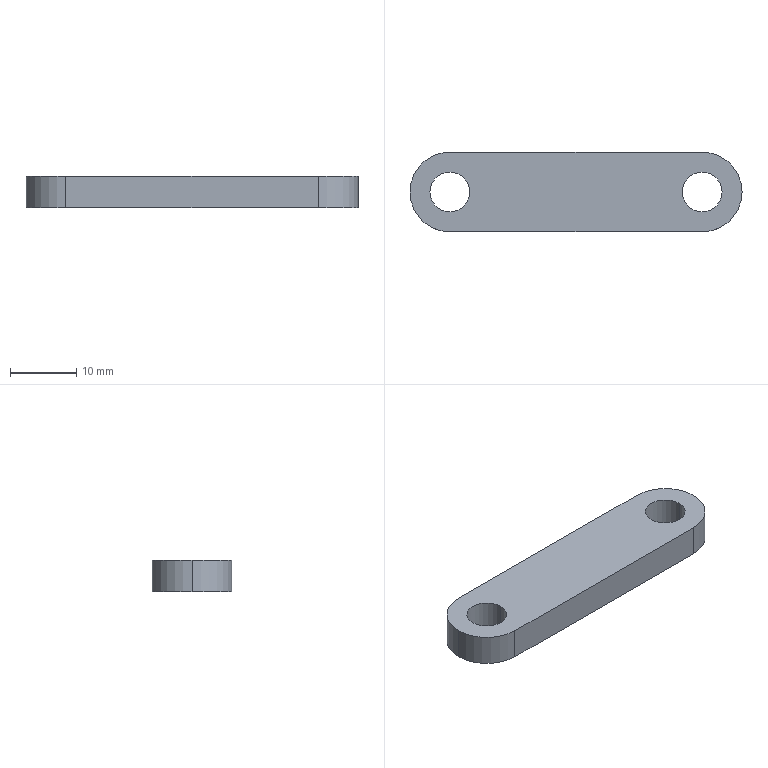Part | STEP file | Ngam kep 5 | 1 solid | 12 faces | box 50 x 12 x 4.8 mm | volume 2460 mm3 | cylinder 8 | plane 4 | commonest cylinder face diameters 6 x4 12 x4
STEP:
#1=CARTESIAN_POINT('',(0.,0.,0.));
#2=DIRECTION('',(0.,0.,1.));
#3=DIRECTION('',(1.,0.,0.));
#4=AXIS2_PLACEMENT_3D('',#1,#2,#3);
#5=CARTESIAN_POINT('',(16.,0.,4.8));
#6=VERTEX_POINT('',#5);
#7=CARTESIAN_POINT('',(16.,0.,0.));
#8=VERTEX_POINT('',#7);
#9=CARTESIAN_POINT('',(16.,0.,4.8));
#10=DIRECTION('',(0.,0.,-1.));
#11=VECTOR('',#10,1.);
#12=LINE('',#9,#11);
#13=CARTESIAN_POINT('',(19.,0.,4.8));
#14=DIRECTION('',(0.,0.,-1.));
#15=DIRECTION('',(-1.,0.,0.));
#16=AXIS2_PLACEMENT_3D('',#13,#14,#15);
#17=CYLINDRICAL_SURFACE('',#16,3.);
#18=CARTESIAN_POINT('',(6.283,0.));
#19=DIRECTION('',(0.,1.));
#20=VECTOR('',#19,1.);
#21=LINE('',#18,#20);
#22=(GEOMETRIC_REPRESENTATION_CONTEXT(2)PARAMETRIC_REPRESENTATION_CONTEXT()REPRESENTATION_CONTEXT('',''));
#23=DEFINITIONAL_REPRESENTATION('',(#21),#22);
#24=PCURVE('',#17,#23);
#25=CARTESIAN_POINT('',(19.,0.,4.8));
#26=DIRECTION('',(0.,0.,-1.));
#27=DIRECTION('',(-1.,0.,0.));
#28=AXIS2_PLACEMENT_3D('',#25,#26,#27);
#29=CYLINDRICAL_SURFACE('',#28,3.);
#30=CARTESIAN_POINT('',(0.,0.));
#31=DIRECTION('',(0.,1.));
#32=VECTOR('',#31,1.);
#33=LINE('',#30,#32);
#34=(GEOMETRIC_REPRESENTATION_CONTEXT(2)PARAMETRIC_REPRESENTATION_CONTEXT()REPRESENTATION_CONTEXT('',''));
#35=DEFINITIONAL_REPRESENTATION('',(#33),#34);
#36=PCURVE('',#29,#35);
#37=SURFACE_CURVE('',#12,(#24,#36),.PCURVE_S1.);
#38=EDGE_CURVE('',#6,#8,#37,.T.);
#39=ORIENTED_EDGE('',*,*,#38,.T.);
#40=CARTESIAN_POINT('',(22.,0.,0.));
#41=VERTEX_POINT('',#40);
#42=CARTESIAN_POINT('',(19.,0.,0.));
#43=DIRECTION('',(0.,0.,1.));
#44=DIRECTION('',(1.,0.,0.));
#45=AXIS2_PLACEMENT_3D('',#42,#43,#44);
#46=CIRCLE('',#45,3.);
#47=CARTESIAN_POINT('',(9.425,4.8));
#48=DIRECTION('',(-1.,0.));
#49=VECTOR('',#48,1.);
#50=LINE('',#47,#49);
#51=(GEOMETRIC_REPRESENTATION_CONTEXT(2)PARAMETRIC_REPRESENTATION_CONTEXT()REPRESENTATION_CONTEXT('',''));
#52=DEFINITIONAL_REPRESENTATION('',(#50),#51);
#53=PCURVE('',#17,#52);
#54=CARTESIAN_POINT('',(0.,0.,0.));
#55=DIRECTION('',(0.,0.,-1.));
#56=DIRECTION('',(-1.,0.,0.));
#57=AXIS2_PLACEMENT_3D('',#54,#55,#56);
#58=PLANE('',#57);
#59=CARTESIAN_POINT('',(-22.,0.));
#60=CARTESIAN_POINT('',(-22.,5.196));
#61=CARTESIAN_POINT('',(-17.5,2.598));
#62=CARTESIAN_POINT('',(-13.,0.));
#63=CARTESIAN_POINT('',(-17.5,-2.598));
#64=CARTESIAN_POINT('',(-22.,-5.196));
#65=CARTESIAN_POINT('',(-22.,0.));
#66=(BOUNDED_CURVE()B_SPLINE_CURVE(2,(#59,#60,#61,#62,#63,#64,#65),.UNSPECIFIED.,.T.,.F.)B_SPLINE_CURVE_WITH_KNOTS((1,2,2,2,2,1),(-2.094,0.,2.094,4.189,6.283,8.378),.UNSPECIFIED.)CURVE()GEOMETRIC_REPRESENTATION_ITEM()RATIONAL_B_SPLINE_CURVE((1.,0.5,1.,0.5,1.,0.5,1.))REPRESENTATION_ITEM(''));
#67=(GEOMETRIC_REPRESENTATION_CONTEXT(2)PARAMETRIC_REPRESENTATION_CONTEXT()REPRESENTATION_CONTEXT('',''));
#68=DEFINITIONAL_REPRESENTATION('',(#66),#67);
#69=PCURVE('',#58,#68);
#70=SURFACE_CURVE('',#46,(#53,#69),.PCURVE_S1.);
#71=EDGE_CURVE('',#8,#41,#70,.T.);
#72=ORIENTED_EDGE('',*,*,#71,.T.);
#73=CARTESIAN_POINT('',(22.,0.,4.8));
#74=VERTEX_POINT('',#73);
#75=CARTESIAN_POINT('',(22.,0.,4.8));
#76=DIRECTION('',(0.,0.,-1.));
#77=VECTOR('',#76,1.);
#78=LINE('',#75,#77);
#79=CARTESIAN_POINT('',(3.142,0.));
#80=DIRECTION('',(0.,1.));
#81=VECTOR('',#80,1.);
#82=LINE('',#79,#81);
#83=(GEOMETRIC_REPRESENTATION_CONTEXT(2)PARAMETRIC_REPRESENTATION_CONTEXT()REPRESENTATION_CONTEXT('',''));
#84=DEFINITIONAL_REPRESENTATION('',(#82),#83);
#85=PCURVE('',#17,#84);
#86=CARTESIAN_POINT('',(3.142,0.));
#87=DIRECTION('',(0.,1.));
#88=VECTOR('',#87,1.);
#89=LINE('',#86,#88);
#90=(GEOMETRIC_REPRESENTATION_CONTEXT(2)PARAMETRIC_REPRESENTATION_CONTEXT()REPRESENTATION_CONTEXT('',''));
#91=DEFINITIONAL_REPRESENTATION('',(#89),#90);
#92=PCURVE('',#29,#91);
#93=SURFACE_CURVE('',#78,(#85,#92),.PCURVE_S1.);
#94=EDGE_CURVE('',#74,#41,#93,.T.);
#95=ORIENTED_EDGE('',*,*,#94,.F.);
#96=CARTESIAN_POINT('',(19.,0.,4.8));
#97=DIRECTION('',(0.,0.,1.));
#98=DIRECTION('',(1.,0.,0.));
#99=AXIS2_PLACEMENT_3D('',#96,#97,#98);
#100=CIRCLE('',#99,3.);
#101=CARTESIAN_POINT('',(9.425,0.));
#102=DIRECTION('',(-1.,0.));
#103=VECTOR('',#102,1.);
#104=LINE('',#101,#103);
#105=(GEOMETRIC_REPRESENTATION_CONTEXT(2)PARAMETRIC_REPRESENTATION_CONTEXT()REPRESENTATION_CONTEXT('',''));
#106=DEFINITIONAL_REPRESENTATION('',(#104),#105);
#107=PCURVE('',#17,#106);
#108=CARTESIAN_POINT('',(0.,0.,4.8));
#109=DIRECTION('',(0.,0.,-1.));
#110=DIRECTION('',(-1.,0.,0.));
#111=AXIS2_PLACEMENT_3D('',#108,#109,#110);
#112=PLANE('',#111);
#113=CARTESIAN_POINT('',(-22.,0.));
#114=CARTESIAN_POINT('',(-22.,5.196));
#115=CARTESIAN_POINT('',(-17.5,2.598));
#116=CARTESIAN_POINT('',(-13.,0.));
#117=CARTESIAN_POINT('',(-17.5,-2.598));
#118=CARTESIAN_POINT('',(-22.,-5.196));
#119=CARTESIAN_POINT('',(-22.,0.));
#120=(BOUNDED_CURVE()B_SPLINE_CURVE(2,(#113,#114,#115,#116,#117,#118,#119),.UNSPECIFIED.,.T.,.F.)B_SPLINE_CURVE_WITH_KNOTS((1,2,2,2,2,1),(-2.094,0.,2.094,4.189,6.283,8.378),.UNSPECIFIED.)CURVE()GEOMETRIC_REPRESENTATION_ITEM()RATIONAL_B_SPLINE_CURVE((1.,0.5,1.,0.5,1.,0.5,1.))REPRESENTATION_ITEM(''));
#121=(GEOMETRIC_REPRESENTATION_CONTEXT(2)PARAMETRIC_REPRESENTATION_CONTEXT()REPRESENTATION_CONTEXT('',''));
#122=DEFINITIONAL_REPRESENTATION('',(#120),#121);
#123=PCURVE('',#112,#122);
#124=SURFACE_CURVE('',#100,(#107,#123),.PCURVE_S1.);
#125=EDGE_CURVE('',#6,#74,#124,.T.);
#126=ORIENTED_EDGE('',*,*,#125,.F.);
#127=EDGE_LOOP('',(#39,#72,#95,#126));
#128=FACE_BOUND('',#127,.F.);
#129=ADVANCED_FACE('',(#128),#17,.F.);
#130=CARTESIAN_POINT('',(-22.,0.,4.8));
#131=VERTEX_POINT('',#130);
#132=CARTESIAN_POINT('',(-22.,0.,0.));
#133=VERTEX_POINT('',#132);
#134=CARTESIAN_POINT('',(-22.,0.,4.8));
#135=DIRECTION('',(0.,0.,-1.));
#136=VECTOR('',#135,1.);
#137=LINE('',#134,#136);
#138=CARTESIAN_POINT('',(-19.,0.,4.8));
#139=DIRECTION('',(0.,0.,-1.));
#140=DIRECTION('',(-1.,0.,0.));
#141=AXIS2_PLACEMENT_3D('',#138,#139,#140);
#142=CYLINDRICAL_SURFACE('',#141,3.);
#143=CARTESIAN_POINT('',(6.283,0.));
#144=DIRECTION('',(0.,1.));
#145=VECTOR('',#144,1.);
#146=LINE('',#143,#145);
#147=(GEOMETRIC_REPRESENTATION_CONTEXT(2)PARAMETRIC_REPRESENTATION_CONTEXT()REPRESENTATION_CONTEXT('',''));
#148=DEFINITIONAL_REPRESENTATION('',(#146),#147);
#149=PCURVE('',#142,#148);
#150=CARTESIAN_POINT('',(-19.,0.,4.8));
#151=DIRECTION('',(0.,0.,-1.));
#152=DIRECTION('',(-1.,0.,0.));
#153=AXIS2_PLACEMENT_3D('',#150,#151,#152);
#154=CYLINDRICAL_SURFACE('',#153,3.);
#155=CARTESIAN_POINT('',(0.,0.));
#156=DIRECTION('',(0.,1.));
#157=VECTOR('',#156,1.);
#158=LINE('',#155,#157);
#159=(GEOMETRIC_REPRESENTATION_CONTEXT(2)PARAMETRIC_REPRESENTATION_CONTEXT()REPRESENTATION_CONTEXT('',''));
#160=DEFINITIONAL_REPRESENTATION('',(#158),#159);
#161=PCURVE('',#154,#160);
#162=SURFACE_CURVE('',#137,(#149,#161),.PCURVE_S1.);
#163=EDGE_CURVE('',#131,#133,#162,.T.);
#164=ORIENTED_EDGE('',*,*,#163,.T.);
#165=CARTESIAN_POINT('',(-16.,0.,0.));
#166=VERTEX_POINT('',#165);
#167=CARTESIAN_POINT('',(-19.,0.,0.));
#168=DIRECTION('',(0.,0.,1.));
#169=DIRECTION('',(1.,0.,0.));
#170=AXIS2_PLACEMENT_3D('',#167,#168,#169);
#171=CIRCLE('',#170,3.);
#172=CARTESIAN_POINT('',(9.425,4.8));
#173=DIRECTION('',(-1.,0.));
#174=VECTOR('',#173,1.);
#175=LINE('',#172,#174);
#176=(GEOMETRIC_REPRESENTATION_CONTEXT(2)PARAMETRIC_REPRESENTATION_CONTEXT()REPRESENTATION_CONTEXT('',''));
#177=DEFINITIONAL_REPRESENTATION('',(#175),#176);
#178=PCURVE('',#142,#177);
#179=CARTESIAN_POINT('',(16.,0.));
#180=CARTESIAN_POINT('',(16.,5.196));
#181=CARTESIAN_POINT('',(20.5,2.598));
#182=CARTESIAN_POINT('',(25.,0.));
#183=CARTESIAN_POINT('',(20.5,-2.598));
#184=CARTESIAN_POINT('',(16.,-5.196));
#185=CARTESIAN_POINT('',(16.,0.));
#186=(BOUNDED_CURVE()B_SPLINE_CURVE(2,(#179,#180,#181,#182,#183,#184,#185),.UNSPECIFIED.,.T.,.F.)B_SPLINE_CURVE_WITH_KNOTS((1,2,2,2,2,1),(-2.094,0.,2.094,4.189,6.283,8.378),.UNSPECIFIED.)CURVE()GEOMETRIC_REPRESENTATION_ITEM()RATIONAL_B_SPLINE_CURVE((1.,0.5,1.,0.5,1.,0.5,1.))REPRESENTATION_ITEM(''));
#187=(GEOMETRIC_REPRESENTATION_CONTEXT(2)PARAMETRIC_REPRESENTATION_CONTEXT()REPRESENTATION_CONTEXT('',''));
#188=DEFINITIONAL_REPRESENTATION('',(#186),#187);
#189=PCURVE('',#58,#188);
#190=SURFACE_CURVE('',#171,(#178,#189),.PCURVE_S1.);
#191=EDGE_CURVE('',#133,#166,#190,.T.);
#192=ORIENTED_EDGE('',*,*,#191,.T.);
#193=CARTESIAN_POINT('',(-16.,0.,4.8));
#194=VERTEX_POINT('',#193);
#195=CARTESIAN_POINT('',(-16.,0.,4.8));
#196=DIRECTION('',(0.,0.,-1.));
#197=VECTOR('',#196,1.);
#198=LINE('',#195,#197);
#199=CARTESIAN_POINT('',(3.142,0.));
#200=DIRECTION('',(0.,1.));
#201=VECTOR('',#200,1.);
#202=LINE('',#199,#201);
#203=(GEOMETRIC_REPRESENTATION_CONTEXT(2)PARAMETRIC_REPRESENTATION_CONTEXT()REPRESENTATION_CONTEXT('',''));
#204=DEFINITIONAL_REPRESENTATION('',(#202),#203);
#205=PCURVE('',#142,#204);
#206=CARTESIAN_POINT('',(3.142,0.));
#207=DIRECTION('',(0.,1.));
#208=VECTOR('',#207,1.);
#209=LINE('',#206,#208);
#210=(GEOMETRIC_REPRESENTATION_CONTEXT(2)PARAMETRIC_REPRESENTATION_CONTEXT()REPRESENTATION_CONTEXT('',''));
#211=DEFINITIONAL_REPRESENTATION('',(#209),#210);
#212=PCURVE('',#154,#211);
#213=SURFACE_CURVE('',#198,(#205,#212),.PCURVE_S1.);
#214=EDGE_CURVE('',#194,#166,#213,.T.);
#215=ORIENTED_EDGE('',*,*,#214,.F.);
#216=CARTESIAN_POINT('',(-19.,0.,4.8));
#217=DIRECTION('',(0.,0.,1.));
#218=DIRECTION('',(1.,0.,0.));
#219=AXIS2_PLACEMENT_3D('',#216,#217,#218);
#220=CIRCLE('',#219,3.);
#221=CARTESIAN_POINT('',(9.425,0.));
#222=DIRECTION('',(-1.,0.));
#223=VECTOR('',#222,1.);
#224=LINE('',#221,#223);
#225=(GEOMETRIC_REPRESENTATION_CONTEXT(2)PARAMETRIC_REPRESENTATION_CONTEXT()REPRESENTATION_CONTEXT('',''));
#226=DEFINITIONAL_REPRESENTATION('',(#224),#225);
#227=PCURVE('',#142,#226);
#228=CARTESIAN_POINT('',(16.,0.));
#229=CARTESIAN_POINT('',(16.,5.196));
#230=CARTESIAN_POINT('',(20.5,2.598));
#231=CARTESIAN_POINT('',(25.,0.));
#232=CARTESIAN_POINT('',(20.5,-2.598));
#233=CARTESIAN_POINT('',(16.,-5.196));
#234=CARTESIAN_POINT('',(16.,0.));
#235=(BOUNDED_CURVE()B_SPLINE_CURVE(2,(#228,#229,#230,#231,#232,#233,#234),.UNSPECIFIED.,.T.,.F.)B_SPLINE_CURVE_WITH_KNOTS((1,2,2,2,2,1),(-2.094,0.,2.094,4.189,6.283,8.378),.UNSPECIFIED.)CURVE()GEOMETRIC_REPRESENTATION_ITEM()RATIONAL_B_SPLINE_CURVE((1.,0.5,1.,0.5,1.,0.5,1.))REPRESENTATION_ITEM(''));
#236=(GEOMETRIC_REPRESENTATION_CONTEXT(2)PARAMETRIC_REPRESENTATION_CONTEXT()REPRESENTATION_CONTEXT('',''));
#237=DEFINITIONAL_REPRESENTATION('',(#235),#236);
#238=PCURVE('',#112,#237);
#239=SURFACE_CURVE('',#220,(#227,#238),.PCURVE_S1.);
#240=EDGE_CURVE('',#131,#194,#239,.T.);
#241=ORIENTED_EDGE('',*,*,#240,.F.);
#242=EDGE_LOOP('',(#164,#192,#215,#241));
#243=FACE_BOUND('',#242,.F.);
#244=ADVANCED_FACE('',(#243),#142,.F.);
#245=ORIENTED_EDGE('',*,*,#240,.F.);
#246=CARTESIAN_POINT('',(-19.,0.,4.8));
#247=DIRECTION('',(0.,0.,1.));
#248=DIRECTION('',(1.,0.,0.));
#249=AXIS2_PLACEMENT_3D('',#246,#247,#248);
#250=CIRCLE('',#249,3.);
#251=CARTESIAN_POINT('',(16.,0.));
#252=CARTESIAN_POINT('',(16.,5.196));
#253=CARTESIAN_POINT('',(20.5,2.598));
#254=CARTESIAN_POINT('',(25.,0.));
#255=CARTESIAN_POINT('',(20.5,-2.598));
#256=CARTESIAN_POINT('',(16.,-5.196));
#257=CARTESIAN_POINT('',(16.,0.));
#258=(BOUNDED_CURVE()B_SPLINE_CURVE(2,(#251,#252,#253,#254,#255,#256,#257),.UNSPECIFIED.,.T.,.F.)B_SPLINE_CURVE_WITH_KNOTS((1,2,2,2,2,1),(-2.094,0.,2.094,4.189,6.283,8.378),.UNSPECIFIED.)CURVE()GEOMETRIC_REPRESENTATION_ITEM()RATIONAL_B_SPLINE_CURVE((1.,0.5,1.,0.5,1.,0.5,1.))REPRESENTATION_ITEM(''));
#259=(GEOMETRIC_REPRESENTATION_CONTEXT(2)PARAMETRIC_REPRESENTATION_CONTEXT()REPRESENTATION_CONTEXT('',''));
#260=DEFINITIONAL_REPRESENTATION('',(#258),#259);
#261=PCURVE('',#112,#260);
#262=CARTESIAN_POINT('',(3.142,0.));
#263=DIRECTION('',(-1.,0.));
#264=VECTOR('',#263,1.);
#265=LINE('',#262,#264);
#266=(GEOMETRIC_REPRESENTATION_CONTEXT(2)PARAMETRIC_REPRESENTATION_CONTEXT()REPRESENTATION_CONTEXT('',''));
#267=DEFINITIONAL_REPRESENTATION('',(#265),#266);
#268=PCURVE('',#154,#267);
#269=SURFACE_CURVE('',#250,(#261,#268),.PCURVE_S1.);
#270=EDGE_CURVE('',#194,#131,#269,.T.);
#271=ORIENTED_EDGE('',*,*,#270,.F.);
#272=EDGE_LOOP('',(#245,#271));
#273=FACE_BOUND('',#272,.T.);
#274=CARTESIAN_POINT('',(-19.,6.,4.8));
#275=VERTEX_POINT('',#274);
#276=CARTESIAN_POINT('',(-25.,0.,4.8));
#277=VERTEX_POINT('',#276);
#278=CARTESIAN_POINT('',(-19.,0.,4.8));
#279=DIRECTION('',(0.,0.,1.));
#280=DIRECTION('',(-1.,0.,0.));
#281=AXIS2_PLACEMENT_3D('',#278,#279,#280);
#282=CIRCLE('',#281,6.);
#283=CARTESIAN_POINT('',(25.,0.));
#284=CARTESIAN_POINT('',(25.,-10.392));
#285=CARTESIAN_POINT('',(16.,-5.196));
#286=CARTESIAN_POINT('',(7.,0.));
#287=CARTESIAN_POINT('',(16.,5.196));
#288=CARTESIAN_POINT('',(25.,10.392));
#289=CARTESIAN_POINT('',(25.,0.));
#290=(BOUNDED_CURVE()B_SPLINE_CURVE(2,(#283,#284,#285,#286,#287,#288,#289),.UNSPECIFIED.,.T.,.F.)B_SPLINE_CURVE_WITH_KNOTS((1,2,2,2,2,1),(-2.094,0.,2.094,4.189,6.283,8.378),.UNSPECIFIED.)CURVE()GEOMETRIC_REPRESENTATION_ITEM()RATIONAL_B_SPLINE_CURVE((1.,0.5,1.,0.5,1.,0.5,1.))REPRESENTATION_ITEM(''));
#291=(GEOMETRIC_REPRESENTATION_CONTEXT(2)PARAMETRIC_REPRESENTATION_CONTEXT()REPRESENTATION_CONTEXT('',''));
#292=DEFINITIONAL_REPRESENTATION('',(#290),#291);
#293=PCURVE('',#112,#292);
#294=CARTESIAN_POINT('',(-19.,0.,4.8));
#295=DIRECTION('',(0.,0.,-1.));
#296=DIRECTION('',(-1.,0.,0.));
#297=AXIS2_PLACEMENT_3D('',#294,#295,#296);
#298=CYLINDRICAL_SURFACE('',#297,6.);
#299=CARTESIAN_POINT('',(6.283,0.));
#300=DIRECTION('',(-1.,0.));
#301=VECTOR('',#300,1.);
#302=LINE('',#299,#301);
#303=(GEOMETRIC_REPRESENTATION_CONTEXT(2)PARAMETRIC_REPRESENTATION_CONTEXT()REPRESENTATION_CONTEXT('',''));
#304=DEFINITIONAL_REPRESENTATION('',(#302),#303);
#305=PCURVE('',#298,#304);
#306=SURFACE_CURVE('',#282,(#293,#305),.PCURVE_S1.);
#307=EDGE_CURVE('',#275,#277,#306,.T.);
#308=ORIENTED_EDGE('',*,*,#307,.T.);
#309=CARTESIAN_POINT('',(-19.,-6.,4.8));
#310=VERTEX_POINT('',#309);
#311=CARTESIAN_POINT('',(-19.,0.,4.8));
#312=DIRECTION('',(0.,0.,1.));
#313=DIRECTION('',(-1.,0.,0.));
#314=AXIS2_PLACEMENT_3D('',#311,#312,#313);
#315=CIRCLE('',#314,6.);
#316=CARTESIAN_POINT('',(25.,0.));
#317=CARTESIAN_POINT('',(25.,-10.392));
#318=CARTESIAN_POINT('',(16.,-5.196));
#319=CARTESIAN_POINT('',(7.,0.));
#320=CARTESIAN_POINT('',(16.,5.196));
#321=CARTESIAN_POINT('',(25.,10.392));
#322=CARTESIAN_POINT('',(25.,0.));
#323=(BOUNDED_CURVE()B_SPLINE_CURVE(2,(#316,#317,#318,#319,#320,#321,#322),.UNSPECIFIED.,.T.,.F.)B_SPLINE_CURVE_WITH_KNOTS((1,2,2,2,2,1),(-2.094,0.,2.094,4.189,6.283,8.378),.UNSPECIFIED.)CURVE()GEOMETRIC_REPRESENTATION_ITEM()RATIONAL_B_SPLINE_CURVE((1.,0.5,1.,0.5,1.,0.5,1.))REPRESENTATION_ITEM(''));
#324=(GEOMETRIC_REPRESENTATION_CONTEXT(2)PARAMETRIC_REPRESENTATION_CONTEXT()REPRESENTATION_CONTEXT('',''));
#325=DEFINITIONAL_REPRESENTATION('',(#323),#324);
#326=PCURVE('',#112,#325);
#327=CARTESIAN_POINT('',(-19.,0.,4.8));
#328=DIRECTION('',(0.,0.,-1.));
#329=DIRECTION('',(-1.,0.,0.));
#330=AXIS2_PLACEMENT_3D('',#327,#328,#329);
#331=CYLINDRICAL_SURFACE('',#330,6.);
#332=CARTESIAN_POINT('',(6.283,0.));
#333=DIRECTION('',(-1.,0.));
#334=VECTOR('',#333,1.);
#335=LINE('',#332,#334);
#336=(GEOMETRIC_REPRESENTATION_CONTEXT(2)PARAMETRIC_REPRESENTATION_CONTEXT()REPRESENTATION_CONTEXT('',''));
#337=DEFINITIONAL_REPRESENTATION('',(#335),#336);
#338=PCURVE('',#331,#337);
#339=SURFACE_CURVE('',#315,(#326,#338),.PCURVE_S1.);
#340=EDGE_CURVE('',#277,#310,#339,.T.);
#341=ORIENTED_EDGE('',*,*,#340,.T.);
#342=CARTESIAN_POINT('',(19.,-6.,4.8));
#343=VERTEX_POINT('',#342);
#344=CARTESIAN_POINT('',(25.,-6.,4.8));
#345=DIRECTION('',(1.,0.,0.));
#346=VECTOR('',#345,1.);
#347=LINE('',#344,#346);
#348=CARTESIAN_POINT('',(-25.,-6.));
#349=DIRECTION('',(-1.,0.));
#350=VECTOR('',#349,1.);
#351=LINE('',#348,#350);
#352=(GEOMETRIC_REPRESENTATION_CONTEXT(2)PARAMETRIC_REPRESENTATION_CONTEXT()REPRESENTATION_CONTEXT('',''));
#353=DEFINITIONAL_REPRESENTATION('',(#351),#352);
#354=PCURVE('',#112,#353);
#355=CARTESIAN_POINT('',(25.,-6.,4.8));
#356=DIRECTION('',(0.,1.,0.));
#357=DIRECTION('',(-1.,0.,0.));
#358=AXIS2_PLACEMENT_3D('',#355,#356,#357);
#359=PLANE('',#358);
#360=CARTESIAN_POINT('',(0.,0.));
#361=DIRECTION('',(-1.,0.));
#362=VECTOR('',#361,1.);
#363=LINE('',#360,#362);
#364=(GEOMETRIC_REPRESENTATION_CONTEXT(2)PARAMETRIC_REPRESENTATION_CONTEXT()REPRESENTATION_CONTEXT('',''));
#365=DEFINITIONAL_REPRESENTATION('',(#363),#364);
#366=PCURVE('',#359,#365);
#367=SURFACE_CURVE('',#347,(#354,#366),.PCURVE_S1.);
#368=EDGE_CURVE('',#310,#343,#367,.T.);
#369=ORIENTED_EDGE('',*,*,#368,.T.);
#370=CARTESIAN_POINT('',(25.,0.,4.8));
#371=VERTEX_POINT('',#370);
#372=CARTESIAN_POINT('',(19.,0.,4.8));
#373=DIRECTION('',(0.,0.,1.));
#374=DIRECTION('',(-1.,0.,0.));
#375=AXIS2_PLACEMENT_3D('',#372,#373,#374);
#376=CIRCLE('',#375,6.);
#377=CARTESIAN_POINT('',(-13.,0.));
#378=CARTESIAN_POINT('',(-13.,-10.392));
#379=CARTESIAN_POINT('',(-22.,-5.196));
#380=CARTESIAN_POINT('',(-31.,0.));
#381=CARTESIAN_POINT('',(-22.,5.196));
#382=CARTESIAN_POINT('',(-13.,10.392));
#383=CARTESIAN_POINT('',(-13.,0.));
#384=(BOUNDED_CURVE()B_SPLINE_CURVE(2,(#377,#378,#379,#380,#381,#382,#383),.UNSPECIFIED.,.T.,.F.)B_SPLINE_CURVE_WITH_KNOTS((1,2,2,2,2,1),(-2.094,0.,2.094,4.189,6.283,8.378),.UNSPECIFIED.)CURVE()GEOMETRIC_REPRESENTATION_ITEM()RATIONAL_B_SPLINE_CURVE((1.,0.5,1.,0.5,1.,0.5,1.))REPRESENTATION_ITEM(''));
#385=(GEOMETRIC_REPRESENTATION_CONTEXT(2)PARAMETRIC_REPRESENTATION_CONTEXT()REPRESENTATION_CONTEXT('',''));
#386=DEFINITIONAL_REPRESENTATION('',(#384),#385);
#387=PCURVE('',#112,#386);
#388=CARTESIAN_POINT('',(19.,0.,4.8));
#389=DIRECTION('',(0.,0.,-1.));
#390=DIRECTION('',(-1.,0.,0.));
#391=AXIS2_PLACEMENT_3D('',#388,#389,#390);
#392=CYLINDRICAL_SURFACE('',#391,6.);
#393=CARTESIAN_POINT('',(6.283,0.));
#394=DIRECTION('',(-1.,0.));
#395=VECTOR('',#394,1.);
#396=LINE('',#393,#395);
#397=(GEOMETRIC_REPRESENTATION_CONTEXT(2)PARAMETRIC_REPRESENTATION_CONTEXT()REPRESENTATION_CONTEXT('',''));
#398=DEFINITIONAL_REPRESENTATION('',(#396),#397);
#399=PCURVE('',#392,#398);
#400=SURFACE_CURVE('',#376,(#387,#399),.PCURVE_S1.);
#401=EDGE_CURVE('',#343,#371,#400,.T.);
#402=ORIENTED_EDGE('',*,*,#401,.T.);
#403=CARTESIAN_POINT('',(19.,6.,4.8));
#404=VERTEX_POINT('',#403);
#405=CARTESIAN_POINT('',(19.,0.,4.8));
#406=DIRECTION('',(0.,0.,1.));
#407=DIRECTION('',(-1.,0.,0.));
#408=AXIS2_PLACEMENT_3D('',#405,#406,#407);
#409=CIRCLE('',#408,6.);
#410=CARTESIAN_POINT('',(-13.,0.));
#411=CARTESIAN_POINT('',(-13.,-10.392));
#412=CARTESIAN_POINT('',(-22.,-5.196));
#413=CARTESIAN_POINT('',(-31.,0.));
#414=CARTESIAN_POINT('',(-22.,5.196));
#415=CARTESIAN_POINT('',(-13.,10.392));
#416=CARTESIAN_POINT('',(-13.,0.));
#417=(BOUNDED_CURVE()B_SPLINE_CURVE(2,(#410,#411,#412,#413,#414,#415,#416),.UNSPECIFIED.,.T.,.F.)B_SPLINE_CURVE_WITH_KNOTS((1,2,2,2,2,1),(-2.094,0.,2.094,4.189,6.283,8.378),.UNSPECIFIED.)CURVE()GEOMETRIC_REPRESENTATION_ITEM()RATIONAL_B_SPLINE_CURVE((1.,0.5,1.,0.5,1.,0.5,1.))REPRESENTATION_ITEM(''));
#418=(GEOMETRIC_REPRESENTATION_CONTEXT(2)PARAMETRIC_REPRESENTATION_CONTEXT()REPRESENTATION_CONTEXT('',''));
#419=DEFINITIONAL_REPRESENTATION('',(#417),#418);
#420=PCURVE('',#112,#419);
#421=CARTESIAN_POINT('',(19.,0.,4.8));
#422=DIRECTION('',(0.,0.,-1.));
#423=DIRECTION('',(-1.,0.,0.));
#424=AXIS2_PLACEMENT_3D('',#421,#422,#423);
#425=CYLINDRICAL_SURFACE('',#424,6.);
#426=CARTESIAN_POINT('',(6.283,0.));
#427=DIRECTION('',(-1.,0.));
#428=VECTOR('',#427,1.);
#429=LINE('',#426,#428);
#430=(GEOMETRIC_REPRESENTATION_CONTEXT(2)PARAMETRIC_REPRESENTATION_CONTEXT()REPRESENTATION_CONTEXT('',''));
#431=DEFINITIONAL_REPRESENTATION('',(#429),#430);
#432=PCURVE('',#425,#431);
#433=SURFACE_CURVE('',#409,(#420,#432),.PCURVE_S1.);
#434=EDGE_CURVE('',#371,#404,#433,.T.);
#435=ORIENTED_EDGE('',*,*,#434,.T.);
#436=CARTESIAN_POINT('',(-25.,6.,4.8));
#437=DIRECTION('',(-1.,0.,0.));
#438=VECTOR('',#437,1.);
#439=LINE('',#436,#438);
#440=CARTESIAN_POINT('',(25.,6.));
#441=DIRECTION('',(1.,0.));
#442=VECTOR('',#441,1.);
#443=LINE('',#440,#442);
#444=(GEOMETRIC_REPRESENTATION_CONTEXT(2)PARAMETRIC_REPRESENTATION_CONTEXT()REPRESENTATION_CONTEXT('',''));
#445=DEFINITIONAL_REPRESENTATION('',(#443),#444);
#446=PCURVE('',#112,#445);
#447=CARTESIAN_POINT('',(-25.,6.,4.8));
#448=DIRECTION('',(0.,-1.,0.));
#449=DIRECTION('',(0.,0.,-1.));
#450=AXIS2_PLACEMENT_3D('',#447,#448,#449);
#451=PLANE('',#450);
#452=CARTESIAN_POINT('',(0.,0.));
#453=DIRECTION('',(0.,-1.));
#454=VECTOR('',#453,1.);
#455=LINE('',#452,#454);
#456=(GEOMETRIC_REPRESENTATION_CONTEXT(2)PARAMETRIC_REPRESENTATION_CONTEXT()REPRESENTATION_CONTEXT('',''));
#457=DEFINITIONAL_REPRESENTATION('',(#455),#456);
#458=PCURVE('',#451,#457);
#459=SURFACE_CURVE('',#439,(#446,#458),.PCURVE_S1.);
#460=EDGE_CURVE('',#404,#275,#459,.T.);
#461=ORIENTED_EDGE('',*,*,#460,.T.);
#462=EDGE_LOOP('',(#308,#341,#369,#402,#435,#461));
#463=FACE_BOUND('',#462,.T.);
#464=ORIENTED_EDGE('',*,*,#125,.F.);
#465=CARTESIAN_POINT('',(19.,0.,4.8));
#466=DIRECTION('',(0.,0.,1.));
#467=DIRECTION('',(1.,0.,0.));
#468=AXIS2_PLACEMENT_3D('',#465,#466,#467);
#469=CIRCLE('',#468,3.);
#470=CARTESIAN_POINT('',(-22.,0.));
#471=CARTESIAN_POINT('',(-22.,5.196));
#472=CARTESIAN_POINT('',(-17.5,2.598));
#473=CARTESIAN_POINT('',(-13.,0.));
#474=CARTESIAN_POINT('',(-17.5,-2.598));
#475=CARTESIAN_POINT('',(-22.,-5.196));
#476=CARTESIAN_POINT('',(-22.,0.));
#477=(BOUNDED_CURVE()B_SPLINE_CURVE(2,(#470,#471,#472,#473,#474,#475,#476),.UNSPECIFIED.,.T.,.F.)B_SPLINE_CURVE_WITH_KNOTS((1,2,2,2,2,1),(-2.094,0.,2.094,4.189,6.283,8.378),.UNSPECIFIED.)CURVE()GEOMETRIC_REPRESENTATION_ITEM()RATIONAL_B_SPLINE_CURVE((1.,0.5,1.,0.5,1.,0.5,1.))REPRESENTATION_ITEM(''));
#478=(GEOMETRIC_REPRESENTATION_CONTEXT(2)PARAMETRIC_REPRESENTATION_CONTEXT()REPRESENTATION_CONTEXT('',''));
#479=DEFINITIONAL_REPRESENTATION('',(#477),#478);
#480=PCURVE('',#112,#479);
#481=CARTESIAN_POINT('',(3.142,0.));
#482=DIRECTION('',(-1.,0.));
#483=VECTOR('',#482,1.);
#484=LINE('',#481,#483);
#485=(GEOMETRIC_REPRESENTATION_CONTEXT(2)PARAMETRIC_REPRESENTATION_CONTEXT()REPRESENTATION_CONTEXT('',''));
#486=DEFINITIONAL_REPRESENTATION('',(#484),#485);
#487=PCURVE('',#29,#486);
#488=SURFACE_CURVE('',#469,(#480,#487),.PCURVE_S1.);
#489=EDGE_CURVE('',#74,#6,#488,.T.);
#490=ORIENTED_EDGE('',*,*,#489,.F.);
#491=EDGE_LOOP('',(#464,#490));
#492=FACE_BOUND('',#491,.T.);
#493=ADVANCED_FACE('',(#273,#463,#492),#112,.F.);
#494=ORIENTED_EDGE('',*,*,#191,.T.);
#495=CARTESIAN_POINT('',(-19.,0.,0.));
#496=DIRECTION('',(0.,0.,1.));
#497=DIRECTION('',(1.,0.,0.));
#498=AXIS2_PLACEMENT_3D('',#495,#496,#497);
#499=CIRCLE('',#498,3.);
#500=CARTESIAN_POINT('',(16.,0.));
#501=CARTESIAN_POINT('',(16.,5.196));
#502=CARTESIAN_POINT('',(20.5,2.598));
#503=CARTESIAN_POINT('',(25.,0.));
#504=CARTESIAN_POINT('',(20.5,-2.598));
#505=CARTESIAN_POINT('',(16.,-5.196));
#506=CARTESIAN_POINT('',(16.,0.));
#507=(BOUNDED_CURVE()B_SPLINE_CURVE(2,(#500,#501,#502,#503,#504,#505,#506),.UNSPECIFIED.,.T.,.F.)B_SPLINE_CURVE_WITH_KNOTS((1,2,2,2,2,1),(-2.094,0.,2.094,4.189,6.283,8.378),.UNSPECIFIED.)CURVE()GEOMETRIC_REPRESENTATION_ITEM()RATIONAL_B_SPLINE_CURVE((1.,0.5,1.,0.5,1.,0.5,1.))REPRESENTATION_ITEM(''));
#508=(GEOMETRIC_REPRESENTATION_CONTEXT(2)PARAMETRIC_REPRESENTATION_CONTEXT()REPRESENTATION_CONTEXT('',''));
#509=DEFINITIONAL_REPRESENTATION('',(#507),#508);
#510=PCURVE('',#58,#509);
#511=CARTESIAN_POINT('',(3.142,4.8));
#512=DIRECTION('',(-1.,0.));
#513=VECTOR('',#512,1.);
#514=LINE('',#511,#513);
#515=(GEOMETRIC_REPRESENTATION_CONTEXT(2)PARAMETRIC_REPRESENTATION_CONTEXT()REPRESENTATION_CONTEXT('',''));
#516=DEFINITIONAL_REPRESENTATION('',(#514),#515);
#517=PCURVE('',#154,#516);
#518=SURFACE_CURVE('',#499,(#510,#517),.PCURVE_S1.);
#519=EDGE_CURVE('',#166,#133,#518,.T.);
#520=ORIENTED_EDGE('',*,*,#519,.T.);
#521=EDGE_LOOP('',(#494,#520));
#522=FACE_BOUND('',#521,.T.);
#523=CARTESIAN_POINT('',(-19.,-6.,0.));
#524=VERTEX_POINT('',#523);
#525=CARTESIAN_POINT('',(19.,-6.,0.));
#526=VERTEX_POINT('',#525);
#527=CARTESIAN_POINT('',(25.,-6.,0.));
#528=DIRECTION('',(1.,0.,0.));
#529=VECTOR('',#528,1.);
#530=LINE('',#527,#529);
#531=CARTESIAN_POINT('',(-25.,-6.));
#532=DIRECTION('',(-1.,0.));
#533=VECTOR('',#532,1.);
#534=LINE('',#531,#533);
#535=(GEOMETRIC_REPRESENTATION_CONTEXT(2)PARAMETRIC_REPRESENTATION_CONTEXT()REPRESENTATION_CONTEXT('',''));
#536=DEFINITIONAL_REPRESENTATION('',(#534),#535);
#537=PCURVE('',#58,#536);
#538=CARTESIAN_POINT('',(0.,-4.8));
#539=DIRECTION('',(-1.,0.));
#540=VECTOR('',#539,1.);
#541=LINE('',#538,#540);
#542=(GEOMETRIC_REPRESENTATION_CONTEXT(2)PARAMETRIC_REPRESENTATION_CONTEXT()REPRESENTATION_CONTEXT('',''));
#543=DEFINITIONAL_REPRESENTATION('',(#541),#542);
#544=PCURVE('',#359,#543);
#545=SURFACE_CURVE('',#530,(#537,#544),.PCURVE_S1.);
#546=EDGE_CURVE('',#524,#526,#545,.T.);
#547=ORIENTED_EDGE('',*,*,#546,.F.);
#548=CARTESIAN_POINT('',(-25.,0.,0.));
#549=VERTEX_POINT('',#548);
#550=CARTESIAN_POINT('',(-19.,0.,0.));
#551=DIRECTION('',(0.,0.,-1.));
#552=DIRECTION('',(-1.,0.,0.));
#553=AXIS2_PLACEMENT_3D('',#550,#551,#552);
#554=CIRCLE('',#553,6.);
#555=CARTESIAN_POINT('',(19.,0.));
#556=DIRECTION('',(1.,0.));
#557=AXIS2_PLACEMENT_2D('',#555,#556);
#558=CIRCLE('',#557,6.);
#559=(GEOMETRIC_REPRESENTATION_CONTEXT(2)PARAMETRIC_REPRESENTATION_CONTEXT()REPRESENTATION_CONTEXT('',''));
#560=DEFINITIONAL_REPRESENTATION('',(#558),#559);
#561=PCURVE('',#58,#560);
#562=CARTESIAN_POINT('',(0.,4.8));
#563=DIRECTION('',(1.,0.));
#564=VECTOR('',#563,1.);
#565=LINE('',#562,#564);
#566=(GEOMETRIC_REPRESENTATION_CONTEXT(2)PARAMETRIC_REPRESENTATION_CONTEXT()REPRESENTATION_CONTEXT('',''));
#567=DEFINITIONAL_REPRESENTATION('',(#565),#566);
#568=PCURVE('',#331,#567);
#569=SURFACE_CURVE('',#554,(#561,#568),.PCURVE_S1.);
#570=EDGE_CURVE('',#524,#549,#569,.T.);
#571=ORIENTED_EDGE('',*,*,#570,.T.);
#572=CARTESIAN_POINT('',(-19.,6.,0.));
#573=VERTEX_POINT('',#572);
#574=CARTESIAN_POINT('',(-19.,0.,0.));
#575=DIRECTION('',(0.,0.,-1.));
#576=DIRECTION('',(-1.,0.,0.));
#577=AXIS2_PLACEMENT_3D('',#574,#575,#576);
#578=CIRCLE('',#577,6.);
#579=CARTESIAN_POINT('',(19.,0.));
#580=DIRECTION('',(1.,0.));
#581=AXIS2_PLACEMENT_2D('',#579,#580);
#582=CIRCLE('',#581,6.);
#583=(GEOMETRIC_REPRESENTATION_CONTEXT(2)PARAMETRIC_REPRESENTATION_CONTEXT()REPRESENTATION_CONTEXT('',''));
#584=DEFINITIONAL_REPRESENTATION('',(#582),#583);
#585=PCURVE('',#58,#584);
#586=CARTESIAN_POINT('',(0.,4.8));
#587=DIRECTION('',(1.,0.));
#588=VECTOR('',#587,1.);
#589=LINE('',#586,#588);
#590=(GEOMETRIC_REPRESENTATION_CONTEXT(2)PARAMETRIC_REPRESENTATION_CONTEXT()REPRESENTATION_CONTEXT('',''));
#591=DEFINITIONAL_REPRESENTATION('',(#589),#590);
#592=PCURVE('',#298,#591);
#593=SURFACE_CURVE('',#578,(#585,#592),.PCURVE_S1.);
#594=EDGE_CURVE('',#549,#573,#593,.T.);
#595=ORIENTED_EDGE('',*,*,#594,.T.);
#596=CARTESIAN_POINT('',(19.,6.,0.));
#597=VERTEX_POINT('',#596);
#598=CARTESIAN_POINT('',(-25.,6.,0.));
#599=DIRECTION('',(-1.,0.,0.));
#600=VECTOR('',#599,1.);
#601=LINE('',#598,#600);
#602=CARTESIAN_POINT('',(25.,6.));
#603=DIRECTION('',(1.,0.));
#604=VECTOR('',#603,1.);
#605=LINE('',#602,#604);
#606=(GEOMETRIC_REPRESENTATION_CONTEXT(2)PARAMETRIC_REPRESENTATION_CONTEXT()REPRESENTATION_CONTEXT('',''));
#607=DEFINITIONAL_REPRESENTATION('',(#605),#606);
#608=PCURVE('',#58,#607);
#609=CARTESIAN_POINT('',(4.8,0.));
#610=DIRECTION('',(0.,-1.));
#611=VECTOR('',#610,1.);
#612=LINE('',#609,#611);
#613=(GEOMETRIC_REPRESENTATION_CONTEXT(2)PARAMETRIC_REPRESENTATION_CONTEXT()REPRESENTATION_CONTEXT('',''));
#614=DEFINITIONAL_REPRESENTATION('',(#612),#613);
#615=PCURVE('',#451,#614);
#616=SURFACE_CURVE('',#601,(#608,#615),.PCURVE_S1.);
#617=EDGE_CURVE('',#597,#573,#616,.T.);
#618=ORIENTED_EDGE('',*,*,#617,.F.);
#619=CARTESIAN_POINT('',(25.,0.,0.));
#620=VERTEX_POINT('',#619);
#621=CARTESIAN_POINT('',(19.,0.,0.));
#622=DIRECTION('',(0.,0.,-1.));
#623=DIRECTION('',(-1.,0.,0.));
#624=AXIS2_PLACEMENT_3D('',#621,#622,#623);
#625=CIRCLE('',#624,6.);
#626=CARTESIAN_POINT('',(-19.,0.));
#627=DIRECTION('',(1.,0.));
#628=AXIS2_PLACEMENT_2D('',#626,#627);
#629=CIRCLE('',#628,6.);
#630=(GEOMETRIC_REPRESENTATION_CONTEXT(2)PARAMETRIC_REPRESENTATION_CONTEXT()REPRESENTATION_CONTEXT('',''));
#631=DEFINITIONAL_REPRESENTATION('',(#629),#630);
#632=PCURVE('',#58,#631);
#633=CARTESIAN_POINT('',(0.,4.8));
#634=DIRECTION('',(1.,0.));
#635=VECTOR('',#634,1.);
#636=LINE('',#633,#635);
#637=(GEOMETRIC_REPRESENTATION_CONTEXT(2)PARAMETRIC_REPRESENTATION_CONTEXT()REPRESENTATION_CONTEXT('',''));
#638=DEFINITIONAL_REPRESENTATION('',(#636),#637);
#639=PCURVE('',#425,#638);
#640=SURFACE_CURVE('',#625,(#632,#639),.PCURVE_S1.);
#641=EDGE_CURVE('',#597,#620,#640,.T.);
#642=ORIENTED_EDGE('',*,*,#641,.T.);
#643=CARTESIAN_POINT('',(19.,0.,0.));
#644=DIRECTION('',(0.,0.,-1.));
#645=DIRECTION('',(-1.,0.,0.));
#646=AXIS2_PLACEMENT_3D('',#643,#644,#645);
#647=CIRCLE('',#646,6.);
#648=CARTESIAN_POINT('',(-19.,0.));
#649=DIRECTION('',(1.,0.));
#650=AXIS2_PLACEMENT_2D('',#648,#649);
#651=CIRCLE('',#650,6.);
#652=(GEOMETRIC_REPRESENTATION_CONTEXT(2)PARAMETRIC_REPRESENTATION_CONTEXT()REPRESENTATION_CONTEXT('',''));
#653=DEFINITIONAL_REPRESENTATION('',(#651),#652);
#654=PCURVE('',#58,#653);
#655=CARTESIAN_POINT('',(0.,4.8));
#656=DIRECTION('',(1.,0.));
#657=VECTOR('',#656,1.);
#658=LINE('',#655,#657);
#659=(GEOMETRIC_REPRESENTATION_CONTEXT(2)PARAMETRIC_REPRESENTATION_CONTEXT()REPRESENTATION_CONTEXT('',''));
#660=DEFINITIONAL_REPRESENTATION('',(#658),#659);
#661=PCURVE('',#392,#660);
#662=SURFACE_CURVE('',#647,(#654,#661),.PCURVE_S1.);
#663=EDGE_CURVE('',#620,#526,#662,.T.);
#664=ORIENTED_EDGE('',*,*,#663,.T.);
#665=EDGE_LOOP('',(#547,#571,#595,#618,#642,#664));
#666=FACE_BOUND('',#665,.T.);
#667=ORIENTED_EDGE('',*,*,#71,.T.);
#668=CARTESIAN_POINT('',(19.,0.,0.));
#669=DIRECTION('',(0.,0.,1.));
#670=DIRECTION('',(1.,0.,0.));
#671=AXIS2_PLACEMENT_3D('',#668,#669,#670);
#672=CIRCLE('',#671,3.);
#673=CARTESIAN_POINT('',(-22.,0.));
#674=CARTESIAN_POINT('',(-22.,5.196));
#675=CARTESIAN_POINT('',(-17.5,2.598));
#676=CARTESIAN_POINT('',(-13.,0.));
#677=CARTESIAN_POINT('',(-17.5,-2.598));
#678=CARTESIAN_POINT('',(-22.,-5.196));
#679=CARTESIAN_POINT('',(-22.,0.));
#680=(BOUNDED_CURVE()B_SPLINE_CURVE(2,(#673,#674,#675,#676,#677,#678,#679),.UNSPECIFIED.,.T.,.F.)B_SPLINE_CURVE_WITH_KNOTS((1,2,2,2,2,1),(-2.094,0.,2.094,4.189,6.283,8.378),.UNSPECIFIED.)CURVE()GEOMETRIC_REPRESENTATION_ITEM()RATIONAL_B_SPLINE_CURVE((1.,0.5,1.,0.5,1.,0.5,1.))REPRESENTATION_ITEM(''));
#681=(GEOMETRIC_REPRESENTATION_CONTEXT(2)PARAMETRIC_REPRESENTATION_CONTEXT()REPRESENTATION_CONTEXT('',''));
#682=DEFINITIONAL_REPRESENTATION('',(#680),#681);
#683=PCURVE('',#58,#682);
#684=CARTESIAN_POINT('',(3.142,4.8));
#685=DIRECTION('',(-1.,0.));
#686=VECTOR('',#685,1.);
#687=LINE('',#684,#686);
#688=(GEOMETRIC_REPRESENTATION_CONTEXT(2)PARAMETRIC_REPRESENTATION_CONTEXT()REPRESENTATION_CONTEXT('',''));
#689=DEFINITIONAL_REPRESENTATION('',(#687),#688);
#690=PCURVE('',#29,#689);
#691=SURFACE_CURVE('',#672,(#683,#690),.PCURVE_S1.);
#692=EDGE_CURVE('',#41,#8,#691,.T.);
#693=ORIENTED_EDGE('',*,*,#692,.T.);
#694=EDGE_LOOP('',(#667,#693));
#695=FACE_BOUND('',#694,.T.);
#696=ADVANCED_FACE('',(#522,#666,#695),#58,.T.);
#697=ORIENTED_EDGE('',*,*,#368,.F.);
#698=CARTESIAN_POINT('',(-19.,-6.,4.8));
#699=DIRECTION('',(0.,0.,-1.));
#700=VECTOR('',#699,1.);
#701=LINE('',#698,#700);
#702=CARTESIAN_POINT('',(44.,0.));
#703=DIRECTION('',(0.,-1.));
#704=VECTOR('',#703,1.);
#705=LINE('',#702,#704);
#706=(GEOMETRIC_REPRESENTATION_CONTEXT(2)PARAMETRIC_REPRESENTATION_CONTEXT()REPRESENTATION_CONTEXT('',''));
#707=DEFINITIONAL_REPRESENTATION('',(#705),#706);
#708=PCURVE('',#359,#707);
#709=CARTESIAN_POINT('',(4.712,0.));
#710=DIRECTION('',(0.,1.));
#711=VECTOR('',#710,1.);
#712=LINE('',#709,#711);
#713=(GEOMETRIC_REPRESENTATION_CONTEXT(2)PARAMETRIC_REPRESENTATION_CONTEXT()REPRESENTATION_CONTEXT('',''));
#714=DEFINITIONAL_REPRESENTATION('',(#712),#713);
#715=PCURVE('',#331,#714);
#716=SURFACE_CURVE('',#701,(#708,#715),.PCURVE_S1.);
#717=EDGE_CURVE('',#310,#524,#716,.T.);
#718=ORIENTED_EDGE('',*,*,#717,.T.);
#719=ORIENTED_EDGE('',*,*,#546,.T.);
#720=CARTESIAN_POINT('',(19.,-6.,4.8));
#721=DIRECTION('',(0.,0.,1.));
#722=VECTOR('',#721,1.);
#723=LINE('',#720,#722);
#724=CARTESIAN_POINT('',(6.,0.));
#725=DIRECTION('',(0.,1.));
#726=VECTOR('',#725,1.);
#727=LINE('',#724,#726);
#728=(GEOMETRIC_REPRESENTATION_CONTEXT(2)PARAMETRIC_REPRESENTATION_CONTEXT()REPRESENTATION_CONTEXT('',''));
#729=DEFINITIONAL_REPRESENTATION('',(#727),#728);
#730=PCURVE('',#359,#729);
#731=CARTESIAN_POINT('',(4.712,0.));
#732=DIRECTION('',(0.,-1.));
#733=VECTOR('',#732,1.);
#734=LINE('',#731,#733);
#735=(GEOMETRIC_REPRESENTATION_CONTEXT(2)PARAMETRIC_REPRESENTATION_CONTEXT()REPRESENTATION_CONTEXT('',''));
#736=DEFINITIONAL_REPRESENTATION('',(#734),#735);
#737=PCURVE('',#392,#736);
#738=SURFACE_CURVE('',#723,(#730,#737),.PCURVE_S1.);
#739=EDGE_CURVE('',#526,#343,#738,.T.);
#740=ORIENTED_EDGE('',*,*,#739,.T.);
#741=EDGE_LOOP('',(#697,#718,#719,#740));
#742=FACE_BOUND('',#741,.T.);
#743=ADVANCED_FACE('',(#742),#359,.F.);
#744=ORIENTED_EDGE('',*,*,#617,.T.);
#745=CARTESIAN_POINT('',(-19.,6.,4.8));
#746=DIRECTION('',(0.,0.,1.));
#747=VECTOR('',#746,1.);
#748=LINE('',#745,#747);
#749=CARTESIAN_POINT('',(0.,6.));
#750=DIRECTION('',(-1.,0.));
#751=VECTOR('',#750,1.);
#752=LINE('',#749,#751);
#753=(GEOMETRIC_REPRESENTATION_CONTEXT(2)PARAMETRIC_REPRESENTATION_CONTEXT()REPRESENTATION_CONTEXT('',''));
#754=DEFINITIONAL_REPRESENTATION('',(#752),#753);
#755=PCURVE('',#451,#754);
#756=CARTESIAN_POINT('',(1.571,0.));
#757=DIRECTION('',(0.,-1.));
#758=VECTOR('',#757,1.);
#759=LINE('',#756,#758);
#760=(GEOMETRIC_REPRESENTATION_CONTEXT(2)PARAMETRIC_REPRESENTATION_CONTEXT()REPRESENTATION_CONTEXT('',''));
#761=DEFINITIONAL_REPRESENTATION('',(#759),#760);
#762=PCURVE('',#298,#761);
#763=SURFACE_CURVE('',#748,(#755,#762),.PCURVE_S1.);
#764=EDGE_CURVE('',#573,#275,#763,.T.);
#765=ORIENTED_EDGE('',*,*,#764,.T.);
#766=ORIENTED_EDGE('',*,*,#460,.F.);
#767=CARTESIAN_POINT('',(19.,6.,4.8));
#768=DIRECTION('',(0.,0.,-1.));
#769=VECTOR('',#768,1.);
#770=LINE('',#767,#769);
#771=CARTESIAN_POINT('',(0.,44.));
#772=DIRECTION('',(1.,0.));
#773=VECTOR('',#772,1.);
#774=LINE('',#771,#773);
#775=(GEOMETRIC_REPRESENTATION_CONTEXT(2)PARAMETRIC_REPRESENTATION_CONTEXT()REPRESENTATION_CONTEXT('',''));
#776=DEFINITIONAL_REPRESENTATION('',(#774),#775);
#777=PCURVE('',#451,#776);
#778=CARTESIAN_POINT('',(1.571,0.));
#779=DIRECTION('',(0.,1.));
#780=VECTOR('',#779,1.);
#781=LINE('',#778,#780);
#782=(GEOMETRIC_REPRESENTATION_CONTEXT(2)PARAMETRIC_REPRESENTATION_CONTEXT()REPRESENTATION_CONTEXT('',''));
#783=DEFINITIONAL_REPRESENTATION('',(#781),#782);
#784=PCURVE('',#425,#783);
#785=SURFACE_CURVE('',#770,(#777,#784),.PCURVE_S1.);
#786=EDGE_CURVE('',#404,#597,#785,.T.);
#787=ORIENTED_EDGE('',*,*,#786,.T.);
#788=EDGE_LOOP('',(#744,#765,#766,#787));
#789=FACE_BOUND('',#788,.T.);
#790=ADVANCED_FACE('',(#789),#451,.F.);
#791=ORIENTED_EDGE('',*,*,#519,.T.);
#792=ORIENTED_EDGE('',*,*,#163,.F.);
#793=ORIENTED_EDGE('',*,*,#270,.F.);
#794=ORIENTED_EDGE('',*,*,#214,.T.);
#795=EDGE_LOOP('',(#791,#792,#793,#794));
#796=FACE_BOUND('',#795,.F.);
#797=ADVANCED_FACE('',(#796),#154,.F.);
#798=ORIENTED_EDGE('',*,*,#692,.T.);
#799=ORIENTED_EDGE('',*,*,#38,.F.);
#800=ORIENTED_EDGE('',*,*,#489,.F.);
#801=ORIENTED_EDGE('',*,*,#94,.T.);
#802=EDGE_LOOP('',(#798,#799,#800,#801));
#803=FACE_BOUND('',#802,.F.);
#804=ADVANCED_FACE('',(#803),#29,.F.);
#805=CARTESIAN_POINT('',(-25.,0.,4.8));
#806=DIRECTION('',(0.,0.,-1.));
#807=VECTOR('',#806,1.);
#808=LINE('',#805,#807);
#809=CARTESIAN_POINT('',(0.,0.));
#810=DIRECTION('',(0.,1.));
#811=VECTOR('',#810,1.);
#812=LINE('',#809,#811);
#813=(GEOMETRIC_REPRESENTATION_CONTEXT(2)PARAMETRIC_REPRESENTATION_CONTEXT()REPRESENTATION_CONTEXT('',''));
#814=DEFINITIONAL_REPRESENTATION('',(#812),#813);
#815=PCURVE('',#298,#814);
#816=CARTESIAN_POINT('',(6.283,0.));
#817=DIRECTION('',(0.,1.));
#818=VECTOR('',#817,1.);
#819=LINE('',#816,#818);
#820=(GEOMETRIC_REPRESENTATION_CONTEXT(2)PARAMETRIC_REPRESENTATION_CONTEXT()REPRESENTATION_CONTEXT('',''));
#821=DEFINITIONAL_REPRESENTATION('',(#819),#820);
#822=PCURVE('',#331,#821);
#823=SURFACE_CURVE('',#808,(#815,#822),.PCURVE_S1.);
#824=EDGE_CURVE('',#277,#549,#823,.T.);
#825=ORIENTED_EDGE('',*,*,#824,.F.);
#826=ORIENTED_EDGE('',*,*,#307,.F.);
#827=ORIENTED_EDGE('',*,*,#764,.F.);
#828=ORIENTED_EDGE('',*,*,#594,.F.);
#829=EDGE_LOOP('',(#825,#826,#827,#828));
#830=FACE_BOUND('',#829,.T.);
#831=ADVANCED_FACE('',(#830),#298,.T.);
#832=ORIENTED_EDGE('',*,*,#340,.F.);
#833=ORIENTED_EDGE('',*,*,#824,.T.);
#834=ORIENTED_EDGE('',*,*,#570,.F.);
#835=ORIENTED_EDGE('',*,*,#717,.F.);
#836=EDGE_LOOP('',(#832,#833,#834,#835));
#837=FACE_BOUND('',#836,.T.);
#838=ADVANCED_FACE('',(#837),#331,.T.);
#839=ORIENTED_EDGE('',*,*,#786,.F.);
#840=ORIENTED_EDGE('',*,*,#434,.F.);
#841=CARTESIAN_POINT('',(25.,0.,4.8));
#842=DIRECTION('',(0.,0.,1.));
#843=VECTOR('',#842,1.);
#844=LINE('',#841,#843);
#845=CARTESIAN_POINT('',(3.142,0.));
#846=DIRECTION('',(0.,-1.));
#847=VECTOR('',#846,1.);
#848=LINE('',#845,#847);
#849=(GEOMETRIC_REPRESENTATION_CONTEXT(2)PARAMETRIC_REPRESENTATION_CONTEXT()REPRESENTATION_CONTEXT('',''));
#850=DEFINITIONAL_REPRESENTATION('',(#848),#849);
#851=PCURVE('',#425,#850);
#852=CARTESIAN_POINT('',(3.142,0.));
#853=DIRECTION('',(0.,-1.));
#854=VECTOR('',#853,1.);
#855=LINE('',#852,#854);
#856=(GEOMETRIC_REPRESENTATION_CONTEXT(2)PARAMETRIC_REPRESENTATION_CONTEXT()REPRESENTATION_CONTEXT('',''));
#857=DEFINITIONAL_REPRESENTATION('',(#855),#856);
#858=PCURVE('',#392,#857);
#859=SURFACE_CURVE('',#844,(#851,#858),.PCURVE_S1.);
#860=EDGE_CURVE('',#620,#371,#859,.T.);
#861=ORIENTED_EDGE('',*,*,#860,.F.);
#862=ORIENTED_EDGE('',*,*,#641,.F.);
#863=EDGE_LOOP('',(#839,#840,#861,#862));
#864=FACE_BOUND('',#863,.T.);
#865=ADVANCED_FACE('',(#864),#425,.T.);
#866=ORIENTED_EDGE('',*,*,#401,.F.);
#867=ORIENTED_EDGE('',*,*,#739,.F.);
#868=ORIENTED_EDGE('',*,*,#663,.F.);
#869=ORIENTED_EDGE('',*,*,#860,.T.);
#870=EDGE_LOOP('',(#866,#867,#868,#869));
#871=FACE_BOUND('',#870,.T.);
#872=ADVANCED_FACE('',(#871),#392,.T.);
#873=CLOSED_SHELL('',(#129,#244,#493,#696,#743,#790,#797,#804,#831,#838,#865,#872));
#874=MANIFOLD_SOLID_BREP('',#873);
#875=(LENGTH_UNIT()NAMED_UNIT(*)SI_UNIT(.MILLI.,.METRE.));
#876=UNCERTAINTY_MEASURE_WITH_UNIT(LENGTH_MEASURE(0.0000001),#875,'','');
#877=(NAMED_UNIT(*)PLANE_ANGLE_UNIT()SI_UNIT($,.RADIAN.));
#878=(NAMED_UNIT(*)SI_UNIT($,.STERADIAN.)SOLID_ANGLE_UNIT());
#879=(GEOMETRIC_REPRESENTATION_CONTEXT(3)GLOBAL_UNCERTAINTY_ASSIGNED_CONTEXT((#876))GLOBAL_UNIT_ASSIGNED_CONTEXT((#875,#877,#878))REPRESENTATION_CONTEXT('',''));
#880=ADVANCED_BREP_SHAPE_REPRESENTATION('',(#4,#874),#879);